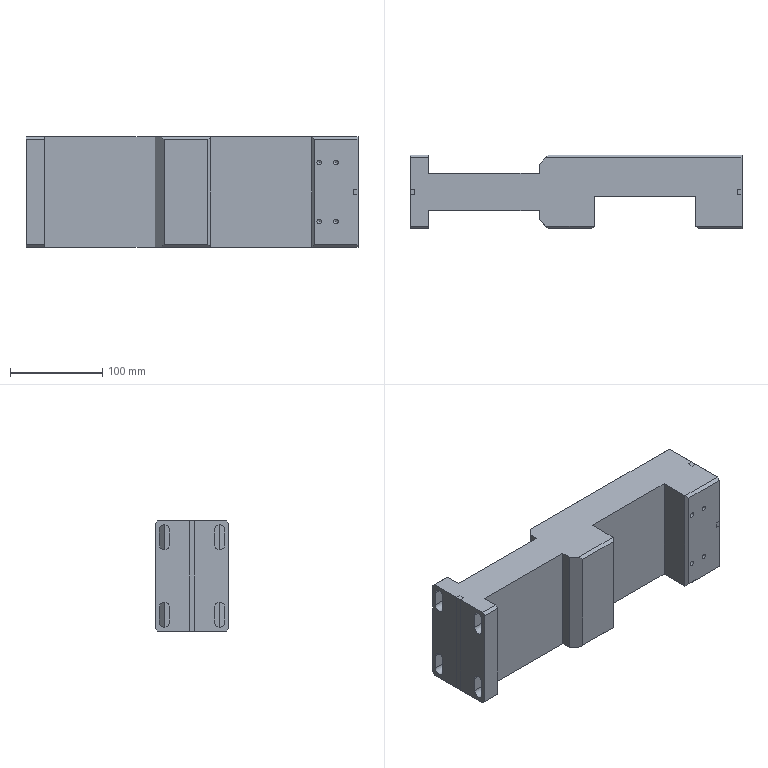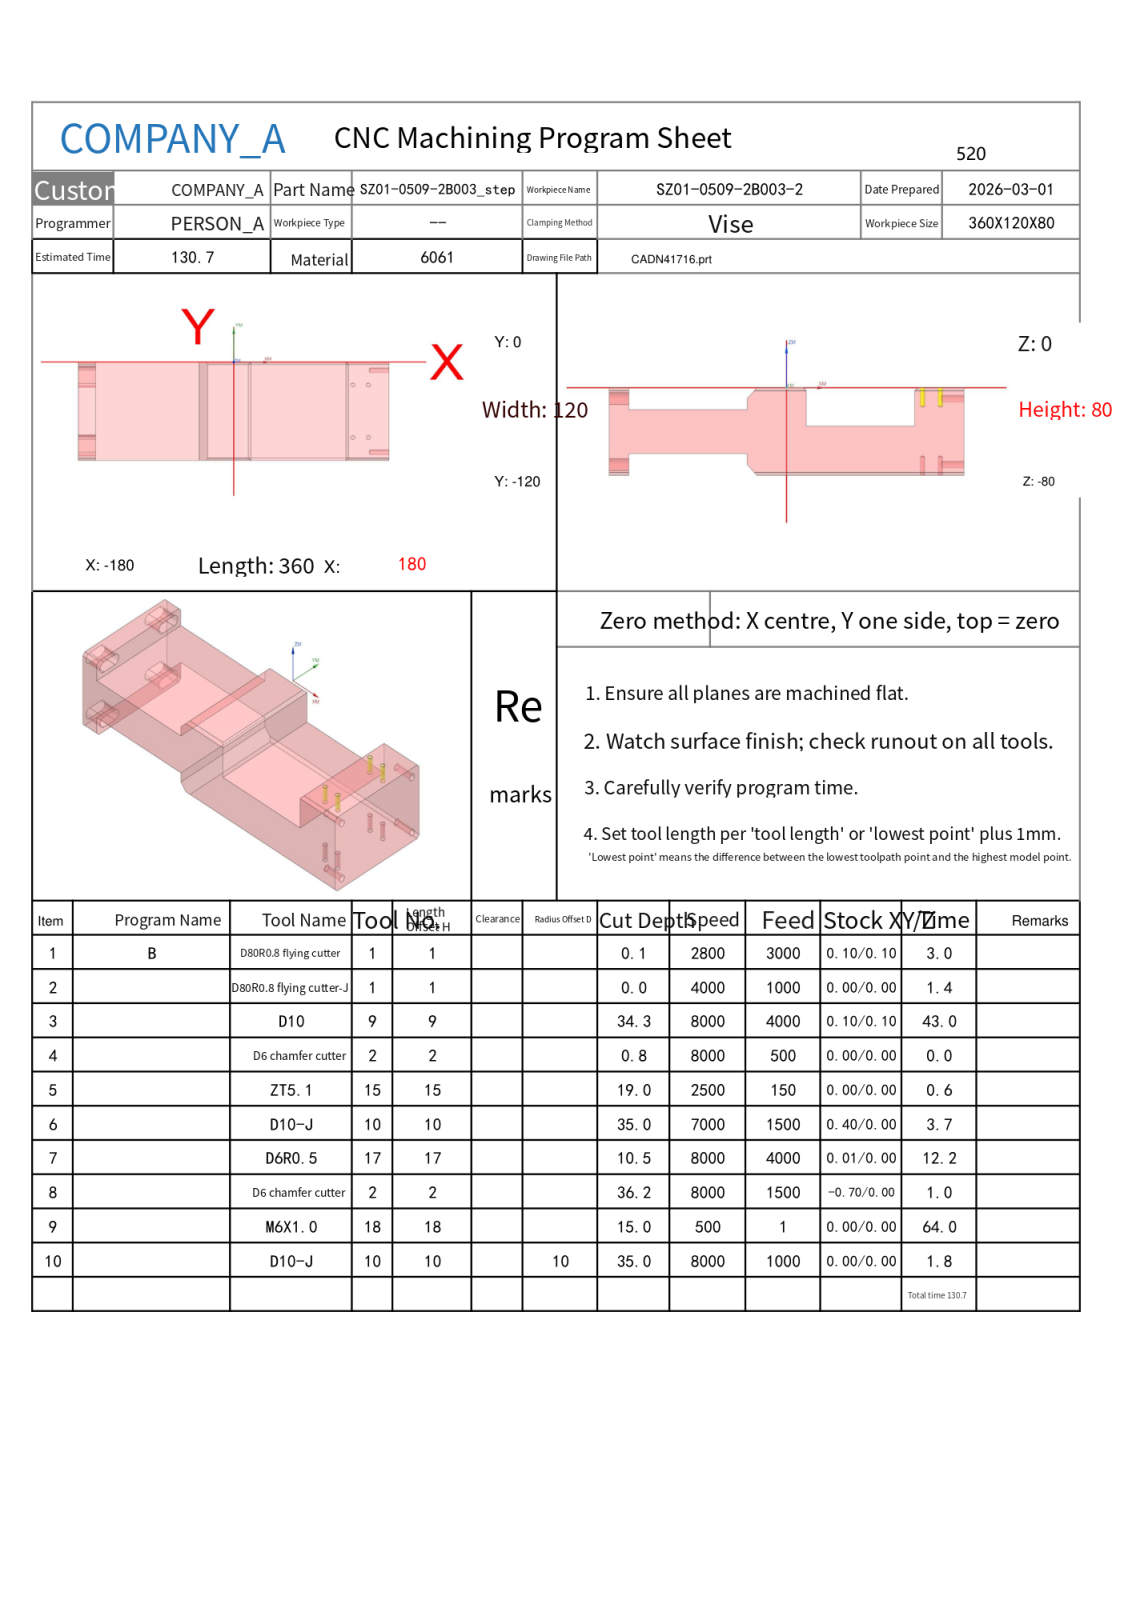NC program | NX | posted by the shop | part box 360 x 80 x 120 mm
Lines 9421 to 12101 of 12457, first 2136 of 2681 lines:
N4 T02 M06
(D6 chamfer cutter  D=6. R=0. H=02 ce=0.00 di=0.10)
G00 G90 G54 X138. Y-28. M03 S8000
G43 H02 Z50.
M08
G98 G81 X138. Y-28. Z-.8 R1. F500.
X156.
Y-92.
X138.
G80
G00 Z50.
G91 G28 Z0.0
M05
M09
G91 G28 Z0.0
M01
N5 T15 M06
(ZT5.1 D=5.1 DR_a=118 H=15)
G00 G90 G54 X138. Y-28. M03 S2500
G43 H15 Z50.
M08
G98 G83 X138. Y-28. Z-19. R1. F150. Q3.
X156.
Y-92.
X138.
G80
G00 Z50.
G91 G28 Z0.0
M05
M09
G91 G28 Z0.0
M01
N6 T10 M06
(D10-J  D=10. R=0. H=10 ce=0.40 di=0.00)
G00 G90 G54 X-98. Y-127. M03 S7000
G43 H10 Z14.5
M08
Z-18.5
G01 Z-20. F1500.
Y-123.
G03 X-100. Y-121. I-2. J0.0
G01 X-153.603
G02 X-154.6 Y-120.003 I.003 J1.
G01 Y.003
G02 X-153.603 Y1. I1. J-.003
G01 X-46.397
G02 X-45.4 Y.003 I-.003 J-1.
G01 Y-120.003
G02 X-46.397 Y-121. I-1. J.003
G01 X-102.086
G02 X-102.792 Y-120.708 I.001 J1.
G01 X-107.207 Y-116.293
G03 X-107.914 Y-116. I-.707 J-.707
G01 X-148.604
G02 X-149.6 Y-115.004 I.004 J1.
G01 Y-4.996
G02 X-148.604 Y-4. I1. J-.004
G01 X-51.396
G02 X-50.4 Y-4.996 I-.004 J-1.
G01 Y-115.004
G02 X-51.396 Y-116. I-1. J.004
G01 X-102.086
G02 X-102.793 Y-115.707 I.001 J1.
G01 X-107.207 Y-111.293
G03 X-107.914 Y-111. I-.707 J-.707
G01 X-143.604
G02 X-144.6 Y-110.004 I.004 J1.
G01 Y-9.996
G02 X-143.604 Y-9. I1. J-.004
G01 X-56.396
G02 X-55.4 Y-9.996 I-.004 J-1.
G01 Y-110.004
G02 X-56.396 Y-111. I-1. J.004
G01 X-102.086
G02 X-102.793 Y-110.707 I.001 J1.
G01 X-107.207 Y-106.293
G03 X-107.914 Y-106. I-.707 J-.707
G01 X-138.604
G02 X-139.6 Y-105.004 I.004 J1.
G01 Y-14.996
G02 X-138.604 Y-14. I1. J-.004
G01 X-61.396
G02 X-60.4 Y-14.996 I-.004 J-1.
G01 Y-105.004
G02 X-61.396 Y-106. I-1. J.004
G01 X-102.086
G02 X-102.793 Y-105.707 I.001 J1.
G01 X-107.207 Y-101.293
G03 X-107.914 Y-101. I-.707 J-.707
G01 X-133.604
G02 X-134.6 Y-100.004 I.004 J1.
G01 Y-19.996
G02 X-133.604 Y-19. I1. J-.004
G01 X-66.396
G02 X-65.4 Y-19.996 I-.004 J-1.
G01 Y-100.004
G02 X-66.396 Y-101. I-1. J.004
G01 X-102.086
G02 X-102.793 Y-100.707 I0.0 J1.
G01 X-107.207 Y-96.293
G03 X-107.914 Y-96. I-.707 J-.707
G01 X-128.605
G02 X-129.6 Y-95.005 I.005 J1.
G01 Y-24.995
G02 X-128.605 Y-24. I1. J-.005
G01 X-71.395
G02 X-70.4 Y-24.995 I-.005 J-1.
G01 Y-95.005
G02 X-71.395 Y-96. I-1. J.005
G01 X-102.086
G02 X-102.793 Y-95.707 I0.0 J1.
G01 X-107.207 Y-91.293
G03 X-107.914 Y-91. I-.707 J-.707
G01 X-123.605
G02 X-124.6 Y-90.005 I.005 J1.
G01 Y-29.995
G02 X-123.605 Y-29. I1. J-.005
G01 X-76.395
G02 X-75.4 Y-29.995 I-.005 J-1.
G01 Y-90.005
G02 X-76.395 Y-91. I-1. J.005
G01 X-102.086
G02 X-102.793 Y-90.707 I0.0 J1.
G01 X-107.207 Y-86.293
G03 X-107.914 Y-86. I-.707 J-.707
G01 X-118.605
G02 X-119.6 Y-85.005 I.005 J1.
G01 Y-34.995
G02 X-118.605 Y-34. I1. J-.005
G01 X-81.395
G02 X-80.4 Y-34.995 I-.005 J-1.
G01 Y-85.005
G02 X-81.395 Y-86. I-1. J.005
G01 X-102.086
G02 X-102.793 Y-85.707 I0.0 J1.
G01 X-107.207 Y-81.293
G03 X-107.914 Y-81. I-.707 J-.707
G01 X-113.605
G02 X-114.6 Y-80.005 I.005 J1.
G01 Y-39.995
G02 X-113.605 Y-39. I1. J-.005
G01 X-86.395
G02 X-85.4 Y-39.995 I-.005 J-1.
G01 Y-80.005
G02 X-86.395 Y-81. I-1. J.005
G01 X-102.086
G02 X-102.793 Y-80.707 I0.0 J1.
G01 X-107.207 Y-76.293
G03 X-107.914 Y-76. I-.707 J-.707
G01 X-108.605
G02 X-109.6 Y-75.005 I.005 J1.
G01 Y-44.995
G02 X-108.605 Y-44. I1. J-.005
G01 X-91.395
G02 X-90.4 Y-44.995 I-.005 J-1.
G01 Y-75.005
G02 X-91.395 Y-76. I-1. J.005
G01 X-101.73
G02 X-102.697 Y-75.255 I0.0 J1.
G01 X-103.706 Y-71.432
G03 X-104.136 Y-70.844 I-.967 J-.256
G02 X-104.6 Y-70.005 I.536 J.844
G01 Y-49.995
G02 X-103.605 Y-49. I1. J-.005
G01 X-96.395
G02 X-95.4 Y-49.995 I-.005 J-1.
G01 Y-70.005
G02 X-96.395 Y-71. I-1. J.005
G01 X-103.605
G02 X-103.827 Y-70.974 I.005 J1.
X-104.542 Y-70.335 I.227 J.974
G03 X-106.427 Y-69.005 I-1.884 J-.67
X-107.097 Y-69.12 I0.0 J-2.
G01 Z-18.5
G00 Z14.5
X77. Y-127.
Z-33.5
G01 Z-35.
Y-123.
G03 X75. Y-121. I-2. J0.0
G01 X26.397
G02 X25.4 Y-120.003 I.003 J1.
G01 Y.003
G02 X26.397 Y1. I1. J-.003
G01 X123.603
G02 X124.6 Y.003 I-.003 J-1.
G01 Y-120.003
G02 X123.603 Y-121. I-1. J.003
G01 X70.
G02 X69.059 Y-120.338 I0.0 J1.
G01 X67.738 Y-116.661
G03 X66.797 Y-116. I-.941 J-.339
G01 X31.396
G02 X30.4 Y-115.004 I.004 J1.
G01 Y-4.996
G02 X31.396 Y-4. I1. J-.004
G01 X118.604
G02 X119.6 Y-4.996 I-.004 J-1.
G01 Y-115.004
G02 X118.604 Y-116. I-1. J.004
G01 X72.914
G02 X72.207 Y-115.707 I.001 J1.
G01 X67.793 Y-111.293
G03 X67.086 Y-111. I-.707 J-.707
G01 X36.396
G02 X35.4 Y-110.004 I.004 J1.
G01 Y-9.996
G02 X36.396 Y-9. I1. J-.004
G01 X113.604
G02 X114.6 Y-9.996 I-.004 J-1.
G01 Y-110.004
G02 X113.604 Y-111. I-1. J.004
G01 X72.914
G02 X72.207 Y-110.707 I.001 J1.
G01 X67.793 Y-106.293
G03 X67.086 Y-106. I-.707 J-.707
G01 X41.396
G02 X40.4 Y-105.004 I.004 J1.
G01 Y-14.996
G02 X41.396 Y-14. I1. J-.004
G01 X108.604
G02 X109.6 Y-14.996 I-.004 J-1.
G01 Y-105.004
G02 X108.604 Y-106. I-1. J.004
G01 X72.914
G02 X72.207 Y-105.707 I0.0 J1.
G01 X67.793 Y-101.293
G03 X67.086 Y-101. I-.707 J-.707
G01 X46.396
G02 X45.4 Y-100.004 I.004 J1.
G01 Y-19.996
G02 X46.396 Y-19. I1. J-.004
G01 X103.604
G02 X104.6 Y-19.996 I-.004 J-1.
G01 Y-100.004
G02 X103.604 Y-101. I-1. J.004
G01 X72.914
G02 X72.207 Y-100.707 I0.0 J1.
G01 X67.793 Y-96.293
G03 X67.086 Y-96. I-.707 J-.707
G01 X51.395
G02 X50.4 Y-95.005 I.005 J1.
G01 Y-24.995
G02 X51.395 Y-24. I1. J-.005
G01 X98.605
G02 X99.6 Y-24.995 I-.005 J-1.
G01 Y-95.005
G02 X98.605 Y-96. I-1. J.005
G01 X72.914
G02 X72.207 Y-95.707 I0.0 J1.
G01 X67.793 Y-91.293
G03 X67.086 Y-91. I-.707 J-.707
G01 X56.395
G02 X55.4 Y-90.005 I.005 J1.
G01 Y-29.995
G02 X56.395 Y-29. I1. J-.005
G01 X93.605
G02 X94.6 Y-29.995 I-.005 J-1.
G01 Y-90.005
G02 X93.605 Y-91. I-1. J.005
G01 X72.914
G02 X72.207 Y-90.707 I0.0 J1.
G01 X67.793 Y-86.293
G03 X67.086 Y-86. I-.707 J-.707
G01 X61.395
G02 X60.4 Y-85.005 I.005 J1.
G01 Y-34.995
G02 X61.395 Y-34. I1. J-.005
G01 X88.605
G02 X89.6 Y-34.995 I-.005 J-1.
G01 Y-85.005
G02 X88.605 Y-86. I-1. J.005
G01 X72.914
G02 X72.207 Y-85.707 I0.0 J1.
G01 X67.793 Y-81.293
G03 X67.086 Y-81. I-.707 J-.707
G01 X66.395
G02 X65.4 Y-80.005 I.005 J1.
G01 Y-39.995
G02 X66.395 Y-39. I1. J-.005
G01 X83.605
G02 X84.6 Y-39.995 I-.005 J-1.
G01 Y-80.005
G02 X83.605 Y-81. I-1. J.005
G01 X73.27
G02 X72.303 Y-80.255 I0.0 J1.
G01 X71.294 Y-76.432
G03 X70.864 Y-75.844 I-.967 J-.256
G02 X70.4 Y-75.005 I.536 J.844
G01 Y-44.995
G02 X71.395 Y-44. I1. J-.005
G01 X78.605
G02 X79.6 Y-44.995 I-.005 J-1.
G01 Y-75.005
G02 X78.605 Y-76. I-1. J.005
G01 X71.395
G02 X71.173 Y-75.974 I.005 J1.
X70.458 Y-75.335 I.227 J.974
G03 X68.573 Y-74.005 I-1.884 J-.67
X67.903 Y-74.12 I0.0 J-2.
G01 Z-33.5
G00 Z14.5
G91 G28 Z0.0
M05
M09
G91 G28 Z0.0
M01
N7 T17 M06
(D6R0.5  D=6. R=0.5 H=17 ce=0.01 di=0.00)
G00 G90 G54 X-32.786 Y-123.363 M03 S8000
G43 H17 Z14.5
M08
Z.429
G01 Z-.071 F4000.
Y-118.232
Y-1.768
X-32.857 Y-1.697 Z-.141
Y-118.303
X-32.927 Y-118.375 Z-.212
X-32.929 Y-118.275
Y-1.725
X-32.927 Y-1.625
X-32.996 Y-1.554 Z-.283
X-33. Y-1.725
Y-118.275
X-32.996 Y-118.446
X-33.068 Y-118.517 Z-.354
X-33.071 Y-118.275
Y-1.725
X-33.068 Y-1.483
X-33.14 Y-1.412 Z-.424
X-33.141 Y-2.722
Y-117.278
X-33.14 Y-118.588
X-33.21 Y-118.66 Z-.495
X-33.212 Y-118.622
Y-1.378
X-33.21 Y-1.34
X-33.28 Y-1.269 Z-.566
X-33.283 Y-1.378
Y-118.622
X-33.28 Y-118.731
X-33.35 Y-118.802 Z-.636
X-33.354 Y-118.622
Y-1.378
X-33.35 Y-1.198
X-33.421 Y-1.127 Z-.707
X-33.424 Y-1.378
Y-118.622
X-33.421 Y-118.873
X-33.494 Y-118.944 Z-.778
X-33.495 Y-117.631
Y-2.369
X-33.494 Y-1.056
X-33.563 Y-.985 Z-.849
X-33.566 Y-1.031
Y-118.969
X-33.563 Y-119.015
X-33.633 Y-119.085 Z-.919
X-33.636 Y-118.969
Y-1.031
X-33.633 Y-.915
X-33.704 Y-.844 Z-.99
X-33.707 Y-1.031
Y-118.969
X-33.704 Y-119.156
X-33.775 Y-119.227 Z-1.061
X-33.778 Y-118.969
Y-1.031
X-33.775 Y-.773
X-33.848 Y-.703 Z-1.131
Y-2.015
Y-117.985
Y-119.297
X-33.917 Y-119.368 Z-1.202
X-33.919 Y-119.316
Y-.684
X-33.917 Y-.632
X-33.987 Y-.562 Z-1.273
X-33.99 Y-.684
Y-119.316
X-33.987 Y-119.438
X-34.057 Y-119.509 Z-1.344
X-34.061 Y-119.316
Y-.684
X-34.057 Y-.491
X-34.129 Y-.42 Z-1.414
X-34.131 Y-1.732
Y-118.268
X-34.129 Y-119.58
X-34.202 Y-119.651 Z-1.485
Y-118.339
Y-1.661
Y-.349
X-34.27 Y-.279 Z-1.556
X-34.273 Y-.337
Y-119.663
X-34.27 Y-119.721
X-34.34 Y-119.792 Z-1.626
X-34.343 Y-119.663
Y-.337
X-34.34 Y-.208
X-34.411 Y-.138 Z-1.697
X-34.414 Y-.337
Y-119.663
X-34.411 Y-119.862
X-34.482 Y-119.932 Z-1.768
X-34.485 Y-118.621
Y-1.379
X-34.482 Y-.068
X-34.555 Y.002 Z-1.838
X-34.556 Y-1.308
Y-118.692
X-34.555 Y-120.002
X-34.624 Y-120.072 Z-1.909
X-34.626 Y-120.009
Y.009
X-34.624 Y.072
X-34.694 Y.142 Z-1.98
X-34.697 Y.009
Y-120.009
X-34.694 Y-120.142
X-34.764 Y-120.212 Z-2.051
X-34.768 Y-120.009
Y.009
X-34.764 Y.212
X-34.836 Y.282 Z-2.121
X-34.838 Y-1.025
Y-118.975
X-34.836 Y-120.282
X-34.909 Y-120.352 Z-2.192
Y-119.046
Y-.954
Y.352
X-34.977 Y.422 Z-2.263
X-34.98 Y.356
Y-120.356
X-34.977 Y-120.422
X-35.047 Y-120.492 Z-2.333
X-35.051 Y-120.356
Y.356
X-35.047 Y.492
X-35.118 Y.562 Z-2.404
X-35.121 Y.356
Y-120.356
X-35.118 Y-120.562
X-35.19 Y-120.632 Z-2.475
X-35.192 Y-119.328
Y-.672
X-35.19 Y.632
X-35.263 Y.702 Z-2.546
Y-.601
Y-119.399
Y-120.702
X-35.331 Y-120.772 Z-2.616
X-35.333 Y-120.703
Y.703
X-35.331 Y.772
X-35.401 Y.842 Z-2.687
X-35.404 Y.703
Y-120.703
X-35.401 Y-120.842
X-35.471 Y-120.912 Z-2.758
X-35.475 Y-120.703
Y.703
X-35.471 Y.912
X-35.543 Y.983 Z-2.828
X-35.546 Y-.318
Y-119.682
X-35.543 Y-120.982
X-35.616 Y-121.05 Z-2.899
Y-119.753
Y-.247
Y1.05
X-35.652 Y1.056 Z-2.934
X-35.686 Y1.061 Z-2.97
X-35.687 Y-.177
Y-119.823
X-35.686 Y-121.061
X-35.722 Y-121.062 Z-3.005
X-35.757 Z-3.041
X-35.758 Y-119.894
Y-.106
X-35.757 Y1.062
X-35.793 Y1.063 Z-3.076
X-35.828 Z-3.111
Y-.035
Y-119.965
Y-121.063
X-35.864 Y-121.064 Z-3.147
X-35.898 Z-3.182
X-35.899 Y-120.
Y0.0
X-35.898 Y1.064
X-35.934 Z-3.217
X-35.969 Y1.065 Z-3.253
X-35.97 Y0.0
Y-120.
X-35.969 Y-121.065
X-36.005 Z-3.288
X-36.04 Z-3.323
X-36.041 Y-120.
Y0.0
X-36.04 Y1.065
X-36.076 Y1.066 Z-3.359
X-36.11 Z-3.394
X-36.111 Y0.0
Y-120.
X-36.11 Y-121.066
X-36.147 Y-121.067 Z-3.429
X-36.181 Z-3.465
X-36.182 Y-120.
Y0.0
X-36.181 Y1.067
X-36.217 Z-3.5
X-36.252 Y1.068 Z-3.536
X-36.253 Y0.0
Y-120.
X-36.252 Y-121.068
X-36.288 Z-3.571
X-36.322 Z-3.606
X-36.323 Y-120.
Y0.0
X-36.322 Y1.068
X-36.359 Y1.069 Z-3.642
X-36.393 Z-3.677
X-36.394 Y0.0
Y-120.
X-36.393 Y-121.069
X-36.429 Z-3.712
X-36.464 Y-121.07 Z-3.748
X-36.465 Y-120.
Y0.0
X-36.464 Y1.07
X-36.5 Z-3.783
X-36.534 Y1.071 Z-3.818
X-36.535 Y0.0
Y-120.
X-36.534 Y-121.071
X-36.571 Z-3.854
X-36.605 Z-3.889
X-36.606 Y-120.
Y0.0
X-36.605 Y1.071
X-36.642 Y1.072 Z-3.924
X-36.676 Z-3.96
X-36.677 Y0.0
Y-120.
X-36.676 Y-121.072
X-36.712 Z-3.995
X-36.746 Y-121.073 Z-4.031
X-36.748 Y-120.
Y0.0
X-36.746 Y1.073
X-36.783 Z-4.066
X-36.817 Y1.074 Z-4.101
X-36.818 Y0.0
Y-120.
X-36.817 Y-121.073
X-36.854 Y-121.074 Z-4.137
X-36.888 Z-4.172
X-36.889 Y-120.
Y0.0
X-36.888 Y1.074
X-36.924 Y1.075 Z-4.207
X-36.958 Z-4.243
X-36.96 Y1.05
Y-121.05
X-36.958 Y-121.075
X-36.995 Z-4.278
X-37.029 Y-121.076 Z-4.313
X-37.03 Y-121.05
Y1.05
X-37.029 Y1.076
X-37.066 Z-4.349
X-37.1 Z-4.384
X-37.101 Y1.05
Y-121.05
X-37.1 Y-121.076
X-37.137 Y-121.077 Z-4.419
X-37.17 Z-4.455
X-37.172 Y-121.05
Y1.05
X-37.17 Y1.077
X-37.207 Z-4.49
X-37.241 Y1.078 Z-4.525
X-37.243 Y1.05
Y-121.05
X-37.241 Y-121.078
X-37.278 Z-4.561
X-37.312 Z-4.596
X-37.313 Y-121.05
Y1.05
X-37.312 Y1.078
X-37.349 Y1.079 Z-4.632
X-37.383 Z-4.667
X-37.384 Y1.05
Y-121.05
X-37.383 Y-121.079
X-37.419 Z-4.702
X-37.453 Z-4.738
X-37.455 Y-121.05
Y1.05
X-37.453 Y1.079
X-37.49 Y1.08 Z-4.773
X-37.524 Z-4.808
X-37.525 Y1.05
Y-121.05
X-37.524 Y-121.08
X-37.561 Z-4.844
X-37.595 Z-4.879
X-37.596 Y-121.05
Y1.05
X-37.595 Y1.08
X-37.632 Y1.081 Z-4.914
X-37.665 Z-4.95
X-37.667 Y1.05
Y-121.05
X-37.665 Y-121.081
X-37.702 Z-4.985
X-37.736 Z-5.02
X-37.738 Y-121.05
Y1.05
X-37.736 Y1.081
X-37.773 Y1.082 Z-5.056
X-37.807 Z-5.091
X-37.808 Y1.05
Y-121.05
X-37.807 Y-121.082
X-37.844 Z-5.127
X-37.877 Z-5.162
X-37.879 Y-121.05
Y1.05
X-37.877 Y1.082
X-37.914 Y1.083 Z-5.197
X-37.948 Z-5.233
X-37.95 Y1.05
Y-121.05
X-37.948 Y-121.083
X-37.985 Z-5.268
X-38.019 Z-5.303
X-38.02 Y-121.05
Y1.05
X-38.019 Y1.083
X-38.056 Y1.084 Z-5.339
X-38.089 Z-5.374
X-38.091 Y1.05
Y-121.05
X-38.089 Y-121.084
X-38.126 Z-5.409
X-38.16 Z-5.445
X-38.162 Y-121.05
Y1.05
X-38.16 Y1.084
X-38.197 Z-5.48
X-38.231 Y1.085 Z-5.515
X-38.233 Y1.05
Y-121.05
X-38.231 Y-121.085
X-38.268 Z-5.551
X-38.302 Z-5.586
X-38.303 Y-121.05
Y1.05
X-38.302 Y1.085
X-38.339 Z-5.622
X-38.372 Y1.086 Z-5.657
X-38.374 Y1.05
Y-121.05
X-38.372 Y-121.086
X-38.409 Z-5.692
X-38.443 Z-5.728
X-38.445 Y-121.05
Y1.05
X-38.443 Y1.086
X-38.48 Z-5.763
X-38.514 Y1.087 Z-5.798
X-38.515 Y1.05
Y-121.05
X-38.514 Y-121.087
X-38.551 Z-5.834
X-38.584 Z-5.869
X-38.586 Y-121.05
Y1.05
X-38.584 Y1.087
X-38.621 Z-5.904
X-38.655 Z-5.94
X-38.657 Y1.05
Y-121.05
X-38.655 Y-121.087
X-38.692 Z-5.975
X-38.726 Z-6.01
X-38.728 Y-120.
Y1.05
X-38.726 Y1.088
X-38.763 Z-6.046
X-38.796 Z-6.081
X-38.798 Y1.05
Y-121.05
X-38.796 Y-121.088
X-38.834 Z-6.116
X-38.867 Z-6.152
X-38.869 Y-121.05
Y1.05
X-38.867 Y1.088
X-38.904 Z-6.187
X-38.938 Z-6.223
X-38.94 Y1.05
Y-121.05
X-38.938 Y-121.088
X-38.975 Z-6.258
X-39.009 Z-6.293
X-39.01 Y-121.05
Y1.05
X-39.009 Y1.088
X-39.046 Z-6.329
X-39.079 Z-6.364
X-39.081 Y1.05
Y-121.05
X-39.079 Y-121.088
X-39.116 Z-6.399
X-39.15 Z-6.435
X-39.152 Y-121.05
Y1.05
X-39.15 Y1.088
X-39.187 Z-6.47
X-39.221 Z-6.505
X-39.222 Y1.05
Y-121.05
X-39.221 Y-121.088
X-39.258 Z-6.541
X-39.291 Y-121.089 Z-6.576
X-39.293 Y-121.05
Y1.05
X-39.291 Y1.088
X-39.329 Z-6.611
X-39.362 Y1.089 Z-6.647
X-39.364 Y1.05
Y-121.05
X-39.362 Y-121.089
X-39.399 Z-6.682
X-39.433 Z-6.718
X-39.435 Y-121.05
Y1.05
X-39.433 Y1.089
X-39.47 Z-6.753
X-39.504 Z-6.788
X-39.505 Y1.05
Y-121.05
X-39.504 Y-121.089
X-39.541 Z-6.824
X-39.574 Z-6.859
X-39.576 Y-121.05
Y1.05
X-39.574 Y1.089
X-39.611 Z-6.894
X-39.645 Z-6.93
X-39.647 Y1.05
Y-121.05
X-39.645 Y-121.089
X-39.682 Z-6.965
X-39.716 Z-7.
X-39.717 Y-121.05
Y1.05
X-39.716 Y1.089
X-39.753 Z-7.036
X-39.786 Z-7.071
X-39.788 Y1.05
Y-121.05
X-39.786 Y-121.089
X-39.824 Z-7.106
X-39.857 Z-7.142
X-39.859 Y-121.05
Y1.05
X-39.857 Y1.089
X-39.894 Z-7.177
X-39.928 Z-7.212
X-39.93 Y1.05
Y-121.05
X-39.928 Y-121.089
X-39.965 Z-7.248
X-39.998 Z-7.283
X-40. Y-121.05
Y1.05
X-39.998 Y1.089
X-40.036 Z-7.319
X-40.069 Z-7.354
X-40.071 Y1.05
Y-121.05
X-40.069 Y-121.089
X-40.106 Z-7.389
X-40.14 Z-7.425
X-40.142 Y-121.05
Y1.05
X-40.14 Y1.089
X-40.177 Z-7.46
X-40.211 Z-7.495
X-40.212 Y1.05
Y-121.05
X-40.211 Y-121.089
X-40.248 Z-7.531
X-40.281 Z-7.566
X-40.283 Y-121.05
Y1.05
X-40.281 Y1.089
X-40.319 Z-7.601
X-40.352 Y1.088 Z-7.637
X-40.354 Y1.05
Y-121.05
X-40.352 Y-121.088
X-40.389 Z-7.672
X-40.423 Z-7.707
X-40.425 Y-121.05
Y1.05
X-40.423 Y1.088
X-40.46 Z-7.743
X-40.493 Z-7.778
X-40.495 Y1.05
Y-121.05
X-40.493 Y-121.088
X-40.531 Z-7.814
X-40.564 Z-7.849
X-40.566 Y-121.05
Y1.05
X-40.564 Y1.088
X-40.601 Z-7.884
X-40.635 Y1.087 Z-7.92
X-40.637 Y1.05
Y-121.05
X-40.635 Y-121.087
X-40.672 Z-7.955
X-40.706 Z-7.99
X-40.707 Y-121.05
Y1.05
X-40.706 Y1.087
X-40.743 Z-8.026
X-40.776 Z-8.061
X-40.778 Y1.05
Y-121.05
X-40.776 Y-121.087
X-40.813 Z-8.096
X-40.847 Y-121.086 Z-8.132
X-40.849 Y-121.05
Y1.05
X-40.847 Y1.087
X-40.884 Z-8.167
X-40.918 Y1.086 Z-8.202
X-40.92 Y1.05
Y-121.05
X-40.918 Y-121.086
X-40.955 Z-8.238
X-40.989 Z-8.273
X-40.99 Y-121.05
Y1.05
X-40.989 Y1.086
X-41.026 Z-8.309
X-41.059 Z-8.344
X-41.061 Y1.05
Y-121.05
X-41.059 Y-121.086
X-41.096 Z-8.379
X-41.13 Z-8.415
X-41.132 Y-121.05
Y1.05
X-41.13 Y1.086
X-41.167 Y1.085 Z-8.45
X-41.201 Z-8.485
X-41.202 Y1.05
Y-121.05
X-41.201 Y-121.085
X-41.238 Z-8.521
X-41.271 Z-8.556
X-41.273 Y-121.05
Y1.05
X-41.271 Y1.085
X-41.308 Z-8.591
X-41.342 Z-8.627
X-41.344 Y1.05
Y-121.05
X-41.342 Y-121.085
X-41.379 Z-8.662
X-41.413 Y-121.084 Z-8.697
X-41.415 Y-121.05
Y1.05
X-41.413 Y1.084
X-41.45 Z-8.733
X-41.484 Z-8.768
X-41.485 Y1.05
Y-121.05
X-41.484 Y-121.084
X-41.521 Z-8.803
X-41.554 Z-8.839
X-41.556 Y-121.05
Y1.05
X-41.554 Y1.084
X-41.591 Y1.083 Z-8.874
X-41.625 Z-8.91
X-41.627 Y1.05
Y-121.05
X-41.625 Y-121.083
X-41.662 Z-8.945
X-41.696 Z-8.98
X-41.697 Y-121.05
Y1.05
X-41.696 Y1.083
X-41.733 Y1.082 Z-9.016
X-41.766 Z-9.051
X-41.768 Y1.05
Y-121.05
X-41.766 Y-121.082
X-41.803 Z-9.086
X-41.837 Z-9.122
X-41.839 Y-121.05
Y1.05
X-41.837 Y1.082
X-41.874 Z-9.157
X-41.908 Y1.081 Z-9.192
X-41.909 Y1.05
Y-121.05
X-41.908 Y-121.081
X-41.945 Z-9.228
X-41.979 Z-9.263
X-41.98 Y-121.05
Y1.05
X-41.979 Y1.081
X-42.016 Z-9.298
X-42.049 Y1.08 Z-9.334
X-42.051 Y1.05
Y-121.05
X-42.049 Y-121.08
X-42.086 Z-9.369
X-42.12 Z-9.405
X-42.122 Y-121.05
Y1.05
X-42.12 Y1.08
X-42.157 Z-9.44
X-42.191 Y1.079 Z-9.475
X-42.192 Y1.05
Y-121.05
X-42.191 Y-121.079
X-42.228 Z-9.511
X-42.262 Z-9.546
X-42.263 Y-121.05
Y1.05
X-42.262 Y1.079
X-42.298 Z-9.581
X-42.332 Y1.078 Z-9.617
X-42.334 Y1.05
Y-121.05
X-42.332 Y-121.078
X-42.369 Z-9.652
X-42.403 Z-9.687
X-42.404 Y-121.05
Y1.05
X-42.403 Y1.078
X-42.44 Z-9.723
X-42.474 Y1.077 Z-9.758
X-42.475 Y1.05
Y-121.05
X-42.474 Y-121.078
X-42.511 Y-121.077 Z-9.793
X-42.545 Z-9.829
X-42.546 Y-121.05
Y1.05
X-42.545 Y1.077
X-42.581 Z-9.864
X-42.616 Y1.076 Z-9.899
X-42.617 Y0.0
Y-120.
X-42.616 Y-121.077
X-42.652 Y-121.076 Z-9.935
X-42.686 Z-9.97
X-42.687 Y-121.05
Y1.05
X-42.686 Y1.076
X-42.723 Z-10.006
X-42.757 Z-10.041
X-42.758 Y1.05
Y-121.05
X-42.757 Y-121.076
X-42.793 Y-121.075 Z-10.076
X-42.827 Z-10.112
X-42.829 Y-121.05
Y1.05
X-42.827 Y1.075
X-42.864 Z-10.147
X-42.898 Z-10.182
Y-121.075
X-42.935 Y-121.074 Z-10.218
X-42.969 Z-10.253
Y1.074
X-43.001 Z-10.284
X-43.031 Z-10.315
Y-121.074
X-43.063 Z-10.346
X-43.092 Y-121.073 Z-10.377
Y1.073
X-43.125 Z-10.407
X-43.154 Z-10.438
Y-121.073
X-43.186 Z-10.469
X-43.216 Z-10.5
Y1.073
G00 Z14.5
G00 G90 X186.221 Y-119.774 M03 S8000
Z14.5
Z.442
G01 Z-.058 F4000.
X181.074
X133.064 Y-119.775
G02 X130.227 Y-116.938 I0.0 J2.837
G01 Y-3.062
G02 X133.064 Y-.225 I2.837 J0.0
G01 X181.074 Y-.226
Y-.196 Z-.087
Y-.168 Z-.116
X133.009 Y-.169
G03 X130.168 Y-3.011 I0.0 J-2.842
G01 Y-116.992
G03 X133.008 Y-119.833 I2.84 J0.0
G01 X181.074 Y-119.832
Y-119.861 Z-.145
Y-119.889 Z-.173
X180. Y-119.891
X132.973
X132.95
G02 X130.109 Y-117.049 I0.0 J2.841
G01 Y-117.002
Y-2.998
Y-2.951
G02 X132.95 Y-.109 I2.841 J0.0
G01 X132.973
X180.
X181.074 Y-.11
Y-.08 Z-.202
X181.075 Y-.052 Z-.231
X180.
X132.915
G03 X130.052 Y-2.915 I0.0 J-2.864
G01 Y-117.085
G03 X132.915 Y-119.948 I2.864 J0.0
G01 X180.
X181.075 Y-119.947
Y-119.977 Z-.26
Y-120.005 Z-.289
X180. Y-120.006
X132.857
G02 X129.994 Y-117.143 I0.0 J2.864
G01 Y-2.857
G02 X132.857 Y.006 I2.864 J0.0
G01 X180.
X181.075 Y.005
Y.035 Z-.318
Y.063 Z-.347
X180. Y.064
X132.799
G03 X129.936 Y-2.799 I0.0 J-2.864
G01 Y-117.201
G03 X132.799 Y-120.064 I2.864 J0.0
G01 X180.
X181.075 Y-120.063
Y-120.093 Z-.376
Y-120.121 Z-.405
X180. Y-120.122
X132.742
G02 X129.878 Y-117.258 I0.0 J2.864
G01 Y-2.742
G02 X132.742 Y.122 I2.864 J0.0
G01 X180.
X181.075 Y.121
X181.076 Y.151 Z-.434
Y.179 Z-.463
X180. Y.18
X132.684
G03 X129.82 Y-2.684 I0.0 J-2.864
G01 Y-117.316
G03 X132.684 Y-120.18 I2.864 J0.0
G01 X180.
X181.076 Y-120.179
Y-120.208 Z-.492
Y-120.236 Z-.52
X180. Y-120.238
X132.626
G02 X129.762 Y-117.374 I0.0 J2.864
G01 Y-2.626
G02 X132.626 Y.238 I2.864 J0.0
G01 X180.
X181.076 Y.237
Y.266 Z-.549
Y.294 Z-.578
X180. Y.295
X132.568
G03 X129.705 Y-2.568 I0.0 J-2.864
G01 Y-117.432
G03 X132.568 Y-120.295 I2.864 J0.0
G01 X180.
X181.076 Y-120.294
Y-120.324 Z-.607
X181.077 Y-120.352 Z-.636
X180. Y-120.353
X132.51
G02 X129.647 Y-117.49 I0.0 J2.864
G01 Y-2.51
G02 X132.51 Y.353 I2.864 J0.0
G01 X180.
X181.077 Y.352
Y.382 Z-.665
Y.41 Z-.694
X180. Y.411
X132.452
G03 X129.589 Y-2.452 I0.0 J-2.864
G01 Y-117.548
G03 X132.452 Y-120.411 I2.864 J0.0
G01 X180.
X181.077 Y-120.41
Y-120.44 Z-.723
Y-120.468 Z-.752
X180. Y-120.469
X132.395
G02 X129.531 Y-117.605 I0.0 J2.864
G01 Y-2.395
G02 X132.395 Y.469 I2.864 J0.0
G01 X180.
X181.077 Y.468
Y.498 Z-.781
Y.526 Z-.81
X180. Y.527
X132.337
G03 X129.473 Y-2.337 I0.0 J-2.864
G01 Y-117.663
G03 X132.337 Y-120.527 I2.864 J0.0
G01 X180.
X181.077 Y-120.526
X181.078 Y-120.556 Z-.839
Y-120.583 Z-.867
X180. Y-120.585
X132.279
G02 X129.415 Y-117.721 I0.0 J2.864
G01 Y-2.279
G02 X132.279 Y.585 I2.864 J0.0
G01 X180.
X181.078 Y.584
Y.613 Z-.896
Y.641 Z-.925
X180. Y.642
X132.221
G03 X129.358 Y-2.221 I0.0 J-2.864
G01 Y-117.779
G03 X132.221 Y-120.642 I2.864 J0.0
G01 X180.
X181.078 Y-120.641
Y-120.671 Z-.954
Y-120.699 Z-.983
X180. Y-120.7
X132.163
G02 X129.3 Y-117.837 I0.0 J2.864
G01 Y-2.163
G02 X132.163 Y.7 I2.864 J0.0
G01 X180.
X181.078 Y.699
Y.729 Z-1.012
Y.757 Z-1.041
X180. Y.758
X132.105
G03 X129.242 Y-2.105 I0.0 J-2.864
G01 Y-117.895
G03 X132.105 Y-120.758 I2.864 J0.0
G01 X180.
X181.078 Y-120.757
X181.079 Y-120.787 Z-1.07
Y-120.815 Z-1.099
X180. Y-120.816
X132.048
G02 X129.184 Y-117.952 I0.0 J2.864
G01 Y-2.048
G02 X132.048 Y.816 I2.864 J0.0
G01 X180.
X181.079 Y.815
Y.845 Z-1.128
Y.873 Z-1.157
X180. Y.874
X131.99
G03 X129.126 Y-1.99 I0.0 J-2.864
G01 Y-118.01
G03 X131.99 Y-120.874 I2.864 J0.0
G01 X180.
X181.079 Y-120.873
Y-120.903 Z-1.186
Y-120.93 Z-1.214
X180. Y-120.932
X131.932
G02 X129.068 Y-118.068 I0.0 J2.864
G01 Y-1.932
G02 X131.932 Y.932 I2.864 J0.0
G01 X180.
X181.079 Y.93
Y.96 Z-1.243
Y.988 Z-1.272
X180. Y.989
X131.874
G03 X129.011 Y-1.874 I0.0 J-2.864
G01 Y-118.126
G03 X131.874 Y-120.989 I2.864 J0.0
G01 X180.
X181.079 Y-120.988
Y-121.018 Z-1.301
Y-121.046 Z-1.33
X180. Y-121.047
X131.816
G02 X128.953 Y-118.184 I0.0 J2.864
G01 Y-1.816
G02 X131.816 Y1.047 I2.864 J0.0
G01 X180.
X181.079 Y1.046
Y1.076 Z-1.359
Y1.104 Z-1.388
X180. Y1.105
X131.759
G03 X128.895 Y-1.759 I0.0 J-2.864
G01 Y-118.241
G03 X131.759 Y-121.105 I2.864 J0.0
G01 X180.
X181.079 Y-121.104
Y-121.134 Z-1.417
Y-121.162 Z-1.446
X180. Y-121.163
X131.701
G02 X128.837 Y-118.299 I0.0 J2.864
G01 Y-1.701
G02 X131.701 Y1.163 I2.864 J0.0
G01 X180.
X181.079 Y1.162
Y1.192 Z-1.475
Y1.22 Z-1.504
X180. Y1.221
X131.643
G03 X128.779 Y-1.643 I0.0 J-2.864
G01 Y-118.357
G03 X131.643 Y-121.221 I2.864 J0.0
G01 X180.
X181.079 Y-121.22
Y-121.25 Z-1.532
Y-121.277 Z-1.561
X180. Y-121.279
X131.585
G02 X128.721 Y-118.415 I0.0 J2.864
G01 Y-1.585
G02 X131.585 Y1.279 I2.864 J0.0
G01 X180.
X181.079 Y1.277
Y1.307 Z-1.59
Y1.335 Z-1.619
X180. Y1.336
X131.527
G03 X128.664 Y-1.527 I0.0 J-2.864
G01 Y-118.473
G03 X131.527 Y-121.336 I2.864 J0.0
G01 X180.
X181.079 Y-121.335
Y-121.365 Z-1.648
Y-121.393 Z-1.677
X180. Y-121.394
X131.469
G02 X128.606 Y-118.531 I0.0 J2.864
G01 Y-1.469
G02 X131.469 Y1.394 I2.864 J0.0
G01 X180.
X181.079 Y1.393
Y1.423 Z-1.706
Y1.451 Z-1.735
X180. Y1.452
X131.412
G03 X128.548 Y-1.412 I0.0 J-2.864
G01 Y-118.588
G03 X131.412 Y-121.452 I2.864 J0.0
G01 X180.
X181.079 Y-121.451
Y-121.481 Z-1.764
Y-121.509 Z-1.793
X180. Y-121.51
X131.354
G02 X128.49 Y-118.646 I0.0 J2.864
G01 Y-1.354
G02 X131.354 Y1.51 I2.864 J0.0
G01 X180.
X181.079 Y1.509
Y1.539 Z-1.822
Y1.567 Z-1.851
X180. Y1.568
X131.296
G03 X128.432 Y-1.296 I0.0 J-2.864
G01 Y-118.704
G03 X131.296 Y-121.568 I2.864 J0.0
G01 X180.
X181.079 Y-121.567
Y-121.597 Z-1.879
Y-121.624 Z-1.908
X180. Y-121.625
X131.238
G02 X128.375 Y-118.762 I0.0 J2.864
G01 Y-1.238
G02 X131.238 Y1.625 I2.864 J0.0
G01 X180.
X181.079 Y1.624
Y1.654 Z-1.937
Y1.682 Z-1.966
X180. Y1.683
X131.18
G03 X128.317 Y-1.18 I0.0 J-2.864
G01 Y-118.82
G03 X131.18 Y-121.683 I2.864 J0.0
G01 X180.
X181.079 Y-121.682
Y-121.712 Z-1.995
Y-121.74 Z-2.024
X180. Y-121.741
X131.122
G02 X128.259 Y-118.878 I0.0 J2.864
G01 Y-1.122
G02 X131.122 Y1.741 I2.864 J0.0
G01 X180.
X181.079 Y1.74
Y1.77 Z-2.053
Y1.798 Z-2.082
X180. Y1.799
X131.065
G03 X128.201 Y-1.065 I0.0 J-2.864
G01 Y-118.935
G03 X131.065 Y-121.799 I2.864 J0.0
G01 X180.
X181.079 Y-121.798
Y-121.828 Z-2.111
Y-121.856 Z-2.14
X180. Y-121.857
X131.007
G02 X128.143 Y-118.993 I0.0 J2.864
G01 Y-1.007
G02 X131.007 Y1.857 I2.864 J0.0
G01 X180.
X181.079 Y1.856
Y1.886 Z-2.169
Y1.914 Z-2.198
X180. Y1.915
X130.949
G03 X128.085 Y-.949 I0.0 J-2.864
G01 Y-119.051
G03 X130.949 Y-121.915 I2.864 J0.0
G01 X180.
X181.079 Y-121.914
Y-121.944 Z-2.226
X181.078 Y-121.971 Z-2.255
X180. Y-121.972
X130.891
G02 X128.028 Y-119.109 I0.0 J2.864
G01 Y-.891
G02 X130.891 Y1.972 I2.864 J0.0
G01 X180.
X181.078 Y1.971
Y2.001 Z-2.284
Y2.029 Z-2.313
X180. Y2.03
X130.833
G03 X127.97 Y-.833 I0.0 J-2.864
G01 Y-119.167
G03 X130.833 Y-122.03 I2.864 J0.0
G01 X180.
X181.078 Y-122.029
Y-122.059 Z-2.342
Y-122.087 Z-2.371
X180. Y-122.088
X130.775
G02 X127.912 Y-119.225 I0.0 J2.864
G01 Y-.775
G02 X130.775 Y2.088 I2.864 J0.0
G01 X180.
X181.078 Y2.087
Y2.117 Z-2.4
Y2.145 Z-2.429
X180. Y2.146
X130.718
G03 X127.854 Y-.718 I0.0 J-2.864
G01 Y-119.282
G03 X130.718 Y-122.146 I2.864 J0.0
G01 X180.
X181.078 Y-122.145
Y-122.175 Z-2.458
X181.077 Y-122.203 Z-2.487
X180. Y-122.204
X130.66
G02 X127.796 Y-119.34 I0.0 J2.864
G01 Y-.66
G02 X130.66 Y2.204 I2.864 J0.0
G01 X180.
X181.077 Y2.203
Y2.233 Z-2.516
Y2.261 Z-2.545
X180. Y2.262
X130.602
G03 X127.738 Y-.602 I0.0 J-2.864
G01 Y-119.398
G03 X130.602 Y-122.262 I2.864 J0.0
G01 X180.
X181.077 Y-122.261
Y-122.291 Z-2.573
Y-122.319 Z-2.602
X180.
X130.544
G02 X127.681 Y-119.456 I0.0 J2.864
G01 Y-.544
G02 X130.544 Y2.319 I2.864 J0.0
G01 X180.
X181.077 Y2.318
Y2.348 Z-2.631
Y2.376 Z-2.66
X180. Y2.377
X130.486
G03 X127.623 Y-.486 I0.0 J-2.864
G01 Y-119.514
G03 X130.486 Y-122.377 I2.864 J0.0
G01 X180.
X181.077
X181.076 Y-122.406 Z-2.689
Y-122.434 Z-2.718
X180. Y-122.435
X130.428
G02 X127.565 Y-119.572 I0.0 J2.864
G01 Y-.428
G02 X130.428 Y2.435 I2.864 J0.0
G01 X180.
X181.076 Y2.434
Y2.464 Z-2.747
Y2.492 Z-2.776
X180. Y2.493
X130.371
G03 X127.507 Y-.371 I0.0 J-2.864
G01 Y-119.629
G03 X130.371 Y-122.493 I2.864 J0.0
G01 X180.
X181.076 Y-122.492
Y-122.522 Z-2.805
Y-122.55 Z-2.834
X180. Y-122.551
X130.313
G02 X127.449 Y-119.687 I0.0 J2.864
G01 Y-.313
G02 X130.313 Y2.551 I2.864 J0.0
G01 X180.
X181.076 Y2.55
X181.075 Y2.58 Z-2.863
Y2.608 Z-2.891
X180. Y2.609
X130.255
G03 X127.391 Y-.255 I0.0 J-2.864
G01 Y-119.745
G03 X130.255 Y-122.609 I2.864 J0.0
G01 X180.
X181.075 Y-122.608
Y-122.638 Z-2.92
Y-122.666 Z-2.949
X180.
X130.197
G02 X127.334 Y-119.803 I0.0 J2.864
G01 Y-.197
G02 X130.197 Y2.666 I2.864 J0.0
G01 X180.
X181.075
Y2.695 Z-2.978
Y2.723 Z-3.007
X180. Y2.724
X130.139
X130.118
G03 X127.275 Y-.118 I0.0 J-2.842
G01 X127.276 Y-.161
Y-119.84
X127.275 Y-119.882
G03 X130.118 Y-122.724 I2.842 J0.0
G01 X130.139
X180.
X181.075
X181.074 Y-122.754 Z-3.036
Y-122.782 Z-3.065
X180.
X130.081
G02 X127.218 Y-119.919 I0.0 J2.864
G01 Y-.081
G02 X130.081 Y2.782 I2.864 J0.0
G01 X180.
X181.074 Y2.781
Y2.811 Z-3.094
Y2.839 Z-3.123
X180. Y2.84
X130.042
X130.002
G03 X127.16 Y-.001 I0.0 J-2.842
G01 Y-.024
Y-119.976
Y-119.999
G03 X130.002 Y-122.84 I2.842 J0.0
G01 X130.042
X180.
X181.074 Y-122.839
Y-122.869 Z-3.152
Y-122.897 Z-3.181
X129.941 Y-122.898
G02 X127.102 Y-120.059 I0.0 J2.839
G01 Y.059
G02 X129.941 Y2.898 I2.839 J0.0
G01 X181.074 Y2.897
Y2.927 Z-3.21
X181.073 Y2.955 Z-3.238
X129.892 Y2.956
G03 X127.044 Y.108 I0.0 J-2.848
G01 Y-120.108
G03 X129.892 Y-122.956 I2.848 J0.0
G01 X181.073 Y-122.955
Y-122.985 Z-3.267
Y-123.013 Z-3.296
X129.828
G02 X126.987 Y-120.172 I0.0 J2.841
G01 Y.172
G02 X129.828 Y3.013 I2.841 J0.0
G01 X181.073
Y3.039 Z-3.322
Y3.064 Z-3.347
X129.777
G03 X126.936 Y.222 I0.0 J-2.841
G01 Y-120.222
G03 X129.777 Y-123.064 I2.841 J0.0
G01 X181.073
Y-123.09 Z-3.373
Y-123.115 Z-3.398
X129.727
G02 X126.891 Y-120.279 I0.0 J2.836
G01 Y.279
G02 X129.727 Y3.115 I2.836 J0.0
G01 X181.073 Y3.114
Y3.138 Z-3.421
X181.072 Y3.16 Z-3.444
X129.675 Y3.161
G03 X126.843 Y.33 I0.0 J-2.831
G01 Y-120.33
G03 X129.675 Y-123.161 I2.831 J0.0
G01 X181.072
Y-123.19 Z-3.472
Y-123.217 Z-3.5
X129.623
G02 X126.786 Y-120.38 I0.0 J2.837
G01 Y.38
G02 X129.622 Y3.217 I2.837 J0.0
G01 X181.072 Y3.216
G00 Z14.5
X-36.348 Y-.23
Z.442
G01 Z-.058
X-31.22
X16.936 Y-.225
G02 X19.773 Y-3.062 I0.0 J-2.837
G01 Y-116.938
G02 X16.936 Y-119.775 I-2.837 J0.0
G01 X-31.22 Y-119.77
X-31.278 Y-119.828 Z-.116
X16.999 Y-119.831
G03 X19.833 Y-116.998 I0.0 J2.833
G01 Y-3.002
G03 X16.999 Y-.169 I-2.833 J0.0
G01 X-31.278 Y-.172
X-31.336 Y-.114 Z-.173
X-31.104 Y-.11
X-30.027 Y-.109
X17.027
G02 X19.891 Y-2.973 I0.0 J-2.864
G01 Y-117.027
G02 X17.027 Y-119.891 I-2.864 J0.0
G01 X-30.027
X-31.104 Y-119.89
X-31.336 Y-119.886
X-31.395 Y-119.945 Z-.231
X-30.085 Y-119.948
X17.085
G03 X19.948 Y-117.085 I0.0 J2.864
G01 Y-2.915
G03 X17.085 Y-.052 I-2.864 J0.0
G01 X-30.085
X-31.395 Y-.055
X-31.453 Y.006 Z-.289
X-30.143
X17.143
G02 X20.006 Y-2.857 I0.0 J-2.864
G01 Y-117.143
G02 X17.143 Y-120.006 I-2.864 J0.0
G01 X-30.143
X-31.453
X-31.511 Y-120.061 Z-.347
X-31.45 Y-120.064
X-30.201
X17.201
G03 X20.064 Y-117.201 I0.0 J2.864
G01 Y-2.799
G03 X17.201 Y.064 I-2.864 J0.0
G01 X-30.201
X-31.45
X-31.511 Y.061
X-31.57 Y.117 Z-.405
X-31.45 Y.121
X-30.258 Y.122
X17.258
G02 X20.122 Y-2.742 I0.0 J-2.864
G01 Y-117.258
G02 X17.258 Y-120.122 I-2.864 J0.0
G01 X-30.258
X-31.45 Y-120.121
X-31.57 Y-120.117
X-31.628 Y-120.175 Z-.463
X-31.45 Y-120.179
X-30.316 Y-120.18
X17.316
G03 X20.18 Y-117.316 I0.0 J2.864
G01 Y-2.684
G03 X17.316 Y.18 I-2.864 J0.0
G01 X-30.316
X-31.45 Y.179
X-31.628 Y.175
X-31.687 Y.233 Z-.52
X-31.45 Y.237
X-30.374 Y.238
X17.374
G02 X20.238 Y-2.626 I0.0 J-2.864
G01 Y-117.374
G02 X17.374 Y-120.238 I-2.864 J0.0
G01 X-30.374
X-31.45 Y-120.237
X-31.686 Y-120.233
X-31.745 Y-120.293 Z-.578
X-30.432 Y-120.295
X17.432
G03 X20.295 Y-117.432 I0.0 J2.864
G01 Y-2.568
G03 X17.432 Y.295 I-2.864 J0.0
G01 X-30.432
X-31.745 Y.293
X-31.803 Y.352 Z-.636
X-30.49 Y.353
X17.49
G02 X20.353 Y-2.51 I0.0 J-2.864
G01 Y-117.49
G02 X17.49 Y-120.353 I-2.864 J0.0
G01 X-30.49
X-31.803 Y-120.352
X-31.861 Y-120.408 Z-.694
X-31.797 Y-120.411
X-30.548
X17.548
G03 X20.411 Y-117.548 I0.0 J2.864
G01 Y-2.452
G03 X17.548 Y.411 I-2.864 J0.0
G01 X-30.548
X-31.797
X-31.861 Y.408
X-31.919 Y.464 Z-.752
X-31.797 Y.469
X-30.605
X17.605
G02 X20.469 Y-2.395 I0.0 J-2.864
G01 Y-117.605
G02 X17.605 Y-120.469 I-2.864 J0.0
G01 X-30.605
X-31.797
X-31.919 Y-120.464
X-31.977 Y-120.522 Z-.81
X-31.797 Y-120.526
X-30.663 Y-120.527
X17.663
G03 X20.527 Y-117.663 I0.0 J2.864
G01 Y-2.337
G03 X17.663 Y.527 I-2.864 J0.0
G01 X-30.663
X-31.797 Y.526
X-31.977 Y.522
X-32.035 Y.58 Z-.867
X-31.797 Y.584
X-30.721 Y.585
X17.721
G02 X20.585 Y-2.279 I0.0 J-2.864
G01 Y-117.721
G02 X17.721 Y-120.585 I-2.864 J0.0
G01 X-30.721
X-31.797 Y-120.584
X-32.035 Y-120.58
X-32.093 Y-120.64 Z-.925
X-30.779 Y-120.642
X17.779
G03 X20.642 Y-117.779 I0.0 J2.864
G01 Y-2.221
G03 X17.779 Y.642 I-2.864 J0.0
G01 X-30.779
X-32.093 Y.64
X-32.151 Y.699 Z-.983
X-30.837 Y.7
X17.837
G02 X20.7 Y-2.163 I0.0 J-2.864
G01 Y-117.837
G02 X17.837 Y-120.7 I-2.864 J0.0
G01 X-30.837
X-32.151 Y-120.699
X-32.209 Y-120.755 Z-1.041
X-32.143 Y-120.758
X-30.895
X17.895
G03 X20.758 Y-117.895 I0.0 J2.864
G01 Y-2.105
G03 X17.895 Y.758 I-2.864 J0.0
G01 X-30.895
X-32.143
X-32.209 Y.755
X-32.267 Y.811 Z-1.099
X-32.143 Y.816
X-30.952
X17.952
G02 X20.816 Y-2.048 I0.0 J-2.864
G01 Y-117.952
G02 X17.952 Y-120.816 I-2.864 J0.0
G01 X-30.952
X-32.143
X-32.267 Y-120.811
X-32.325 Y-120.869 Z-1.157
X-32.143 Y-120.873
X-31.01 Y-120.874
X18.01
G03 X20.874 Y-118.01 I0.0 J2.864
G01 Y-1.99
G03 X18.01 Y.874 I-2.864 J0.0
G01 X-31.01
X-32.143 Y.873
X-32.325 Y.869
X-32.383 Y.927 Z-1.214
X-32.143 Y.931
X-31.068 Y.932
X18.068
G02 X20.932 Y-1.932 I0.0 J-2.864
G01 Y-118.068
G02 X18.068 Y-120.932 I-2.864 J0.0
G01 X-31.068
X-32.143 Y-120.931
X-32.383 Y-120.927
X-32.441 Y-120.987 Z-1.272
X-31.126 Y-120.989
X18.126
G03 X20.989 Y-118.126 I0.0 J2.864
G01 Y-1.874
G03 X18.126 Y.989 I-2.864 J0.0
G01 X-31.126
X-32.441 Y.987
X-32.499 Y1.046 Z-1.33
X-31.184 Y1.047
X18.184
G02 X21.047 Y-1.816 I0.0 J-2.864
G01 Y-118.184
G02 X18.184 Y-121.047 I-2.864 J0.0
G01 X-31.184
X-32.499 Y-121.046
X-32.556 Y-121.102 Z-1.388
X-32.49 Y-121.105
X-31.241
X18.241
G03 X21.105 Y-118.241 I0.0 J2.864
G01 Y-1.759
G03 X18.241 Y1.105 I-2.864 J0.0
G01 X-31.241
X-32.49
X-32.556 Y1.102
X-32.614 Y1.158 Z-1.446
X-32.49 Y1.162
X-31.299 Y1.163
X18.299
G02 X21.163 Y-1.701 I0.0 J-2.864
G01 Y-118.299
G02 X18.299 Y-121.163 I-2.864 J0.0
G01 X-31.299
X-32.49 Y-121.162
X-32.614 Y-121.158
X-32.672 Y-121.216 Z-1.504
X-32.49 Y-121.22
X-31.357 Y-121.221
X18.357
G03 X21.221 Y-118.357 I0.0 J2.864
G01 Y-1.643
G03 X18.357 Y1.221 I-2.864 J0.0
G01 X-31.357
X-32.49 Y1.22
X-32.672 Y1.216
X-32.73 Y1.274 Z-1.561
X-32.49 Y1.278
X-31.415 Y1.279
X18.415
G02 X21.279 Y-1.585 I0.0 J-2.864
G01 Y-118.415
G02 X18.415 Y-121.279 I-2.864 J0.0
G01 X-31.415
X-32.49 Y-121.278
X-32.73 Y-121.274
X-32.788 Y-121.334 Z-1.619
X-31.473 Y-121.336
X18.473
G03 X21.336 Y-118.473 I0.0 J2.864
G01 Y-1.527
G03 X18.473 Y1.336 I-2.864 J0.0
G01 X-31.473
X-32.788 Y1.334
X-32.846 Y1.393 Z-1.677
X-31.531 Y1.394
X18.531
G02 X21.394 Y-1.469 I0.0 J-2.864
G01 Y-118.531
G02 X18.531 Y-121.394 I-2.864 J0.0
G01 X-31.531
X-32.846 Y-121.393
X-32.903 Y-121.449 Z-1.735
X-32.836 Y-121.452
X-31.588
X18.588
G03 X21.452 Y-118.588 I0.0 J2.864
G01 Y-1.412
G03 X18.588 Y1.452 I-2.864 J0.0
G01 X-31.588
X-32.836
X-32.903 Y1.449
X-32.961 Y1.505 Z-1.793
X-32.836 Y1.509
X-31.646 Y1.51
X18.646
G02 X21.51 Y-1.354 I0.0 J-2.864
G01 Y-118.646
G02 X18.646 Y-121.51 I-2.864 J0.0
G01 X-31.646
X-32.836 Y-121.509
X-32.961 Y-121.505
X-33.018 Y-121.563 Z-1.851
X-32.836 Y-121.567
X-31.704 Y-121.568
X18.704
G03 X21.568 Y-118.704 I0.0 J2.864
G01 Y-1.296
G03 X18.704 Y1.568 I-2.864 J0.0
G01 X-31.704
X-32.836 Y1.567
X-33.018 Y1.563
X-33.076 Y1.621 Z-1.908
X-32.836 Y1.625
X-31.762
X18.762
G02 X21.625 Y-1.238 I0.0 J-2.864
G01 Y-118.762
G02 X18.762 Y-121.625 I-2.864 J0.0
G01 X-31.762
X-32.836
X-33.076 Y-121.621
X-33.133 Y-121.681 Z-1.966
X-31.82 Y-121.683
X18.82
G03 X21.683 Y-118.82 I0.0 J2.864
G01 Y-1.18
G03 X18.82 Y1.683 I-2.864 J0.0
G01 X-31.82
X-33.133 Y1.681
X-33.19 Y1.74 Z-2.024
X-31.878 Y1.741
X18.878
G02 X21.741 Y-1.122 I0.0 J-2.864
G01 Y-118.878
G02 X18.878 Y-121.741 I-2.864 J0.0
G01 X-31.878
X-33.19 Y-121.74
X-33.248 Y-121.796 Z-2.082
X-33.183 Y-121.799
X-31.935
X18.935
G03 X21.799 Y-118.935 I0.0 J2.864
G01 Y-1.065
G03 X18.935 Y1.799 I-2.864 J0.0
G01 X-31.935
X-33.183
X-33.248 Y1.796
X-33.305 Y1.852 Z-2.14
X-33.183 Y1.856
X-31.993 Y1.857
X18.993
G02 X21.857 Y-1.007 I0.0 J-2.864
G01 Y-118.993
G02 X18.993 Y-121.857 I-2.864 J0.0
G01 X-31.993
X-33.183 Y-121.856
X-33.305 Y-121.852
X-33.363 Y-121.91 Z-2.198
X-33.183 Y-121.914
X-32.051 Y-121.915
X19.051
G03 X21.915 Y-119.051 I0.0 J2.864
G01 Y-.949
G03 X19.051 Y1.915 I-2.864 J0.0
G01 X-32.051
X-33.183 Y1.914
X-33.363 Y1.91
X-33.42 Y1.968 Z-2.255
X-33.183 Y1.972
X-32.109
X19.109
G02 X21.972 Y-.891 I0.0 J-2.864
G01 Y-119.109
G02 X19.109 Y-121.972 I-2.864 J0.0
G01 X-32.109
X-33.183
X-33.42 Y-121.968
X-33.478 Y-122.028 Z-2.313
X-32.167 Y-122.03
X19.167
G03 X22.03 Y-119.167 I0.0 J2.864
G01 Y-.833
G03 X19.167 Y2.03 I-2.864 J0.0
G01 X-32.167
X-33.478 Y2.028
X-33.535 Y2.087 Z-2.371
X-32.225 Y2.088
X19.225
G02 X22.088 Y-.775 I0.0 J-2.864
G01 Y-119.225
G02 X19.225 Y-122.088 I-2.864 J0.0
G01 X-32.225
X-33.535 Y-122.087
X-33.592 Y-122.143 Z-2.429
X-33.529 Y-122.146
X-32.282
X19.282
G03 X22.146 Y-119.282 I0.0 J2.864
G01 Y-.718
G03 X19.282 Y2.146 I-2.864 J0.0
G01 X-32.282
X-33.529
X-33.592 Y2.143
X-33.65 Y2.199 Z-2.487
X-33.529 Y2.203
X-32.34 Y2.204
X19.34
G02 X22.204 Y-.66 I0.0 J-2.864
G01 Y-119.34
G02 X19.34 Y-122.204 I-2.864 J0.0
G01 X-32.34
X-33.529
X-33.65 Y-122.199
X-33.707 Y-122.257 Z-2.545
X-33.529 Y-122.261
X-32.398 Y-122.262
X19.398
G03 X22.262 Y-119.398 I0.0 J2.864
G01 Y-.602
G03 X19.398 Y2.262 I-2.864 J0.0
G01 X-32.398
X-33.529 Y2.261
X-33.707 Y2.257
X-33.765 Y2.315 Z-2.602
X-33.529 Y2.319
X-32.456
X19.456
G02 X22.319 Y-.544 I0.0 J-2.864
G01 Y-119.456
G02 X19.456 Y-122.319 I-2.864 J0.0
G01 X-32.456
X-33.529
X-33.765 Y-122.315
X-33.822 Y-122.375 Z-2.66
X-32.514 Y-122.377
X19.514
G03 X22.377 Y-119.514 I0.0 J2.864
G01 Y-.486
G03 X19.514 Y2.377 I-2.864 J0.0
G01 X-32.514
X-33.822 Y2.375
X-33.879 Y2.435 Z-2.718
X-32.572
X19.572
G02 X22.435 Y-.428 I0.0 J-2.864
G01 Y-119.572
G02 X19.572 Y-122.435 I-2.864 J0.0
G01 X-32.572
X-33.879
X-33.937 Y-122.49 Z-2.776
X-33.876 Y-122.493
X-32.629
X19.629
G03 X22.493 Y-119.629 I0.0 J2.864
G01 Y-.371
G03 X19.629 Y2.493 I-2.864 J0.0
G01 X-32.629
X-33.876
X-33.937 Y2.49
X-33.994 Y2.546 Z-2.834
X-33.876 Y2.551
X-32.687
X19.687
G02 X22.551 Y-.313 I0.0 J-2.864
G01 Y-119.687
G02 X19.687 Y-122.551 I-2.864 J0.0
G01 X-32.687
X-33.876
X-33.994 Y-122.546
X-34.052 Y-122.604 Z-2.891
X-33.876 Y-122.608
X-32.745 Y-122.609
X19.745
G03 X22.609 Y-119.745 I0.0 J2.864
G01 Y-.255
G03 X19.745 Y2.609 I-2.864 J0.0
G01 X-32.745
X-33.876 Y2.608
X-34.052 Y2.604
X-34.109 Y2.662 Z-2.949
X-33.876 Y2.666
X-32.803
X19.826
G02 X22.666 Y-.174 I0.0 J-2.84
G01 Y-119.826
G02 X19.826 Y-122.666 I-2.84 J0.0
G01 X-32.803
X-33.876
X-34.109 Y-122.662
X-34.167 Y-122.722 Z-3.007
X-32.861 Y-122.724
X19.861
G03 X22.724 Y-119.861 I0.0 J2.864
G01 Y-.139
G03 X19.861 Y2.724 I-2.864 J0.0
G01 X-32.861
X-34.167 Y2.721
X-34.224 Y2.782 Z-3.065
X-32.919
X19.919
G02 X22.782 Y-.081 I0.0 J-2.864
G01 Y-119.919
G02 X19.919 Y-122.782 I-2.864 J0.0
G01 X-32.919
X-34.224
Y-122.811 Z-3.094
X-34.225 Y-122.84 Z-3.123
X-32.976
X19.952
X19.998
G03 X22.84 Y-119.999 I0.0 J2.842
G01 Y-119.976
Y-.024
Y-.001
G03 X19.998 Y2.84 I-2.842 J0.0
G01 X19.952
X-32.976
X-34.225
X-34.224 Y2.869 Z-3.152
X-34.223 Y2.898 Z-3.181
X20.053 Y2.897
G02 X22.898 Y.052 I0.0 J-2.845
G01 Y-120.052
G02 X20.053 Y-122.897 I-2.845 J0.0
G01 X-34.223 Y-122.898
X-34.179 Y-122.954 Z-3.238
X20.108 Y-122.956
G03 X22.956 Y-120.108 I0.0 J2.847
G01 Y.108
G03 X20.108 Y2.956 I-2.847 J0.0
G01 X-34.18 Y2.954
X-34.128 Y3.011 Z-3.296
X20.172 Y3.013
G02 X23.013 Y.172 I0.0 J-2.841
G01 Y-120.172
G02 X20.172 Y-123.013 I-2.841 J0.0
G01 X-34.127 Y-123.011
X-34.082 Y-123.061 Z-3.347
X20.223 Y-123.064
G03 X23.064 Y-120.222 I0.0 J2.841
G01 Y.222
G03 X20.223 Y3.064 I-2.841 J0.0
G01 X-34.082 Y3.061
X-34.036 Y3.112 Z-3.398
X20.273 Y3.115
G02 X23.109 Y.279 I0.0 J-2.836
G01 Y-120.279
G02 X20.273 Y-123.115 I-2.836 J0.0
G01 X-34.036 Y-123.112
X-33.995 Y-123.158 Z-3.444
X20.325 Y-123.161
G03 X23.157 Y-120.33 I0.0 J2.832
G01 Y.33
G03 X20.325 Y3.161 I-2.832 J0.0
G01 X-33.995 Y3.158
X-33.945 Y3.214 Z-3.5
X20.377 Y3.217
G02 X23.214 Y.38 I0.0 J-2.837
G01 Y-120.38
G02 X20.377 Y-123.217 I-2.837 J0.0
G01 X-33.945 Y-123.214
G00 Z14.5
X-153.773 Y-119.771
Z.442
G01 Z-.058
X-158.927 Y-119.772
X-181.074 Y-119.775
Y-119.804 Z-.087
Y-119.833 Z-.116
X-158.926 Y-119.83
Y-119.862 Z-.145
Y-119.888 Z-.173
X-159.076 Y-119.891
X-180.
X-181.074
Y-119.92 Z-.202
X-181.075 Y-119.948 Z-.231
X-180.
X-159.076
X-158.926 Y-119.946
X-158.925 Y-119.977 Z-.26
Y-120.003 Z-.289
X-159.076 Y-120.006
X-180.
X-181.075
Y-120.035 Z-.318
Y-120.064 Z-.347
X-180.
X-159.076
X-158.925 Y-120.061
Y-120.093 Z-.376
Y-120.119 Z-.405
X-159.076 Y-120.122
X-180.
X-181.075
X-181.076 Y-120.151 Z-.434
Y-120.18 Z-.463
X-180.
X-159.076
X-158.924 Y-120.177
Y-120.209 Z-.492
Y-120.235 Z-.52